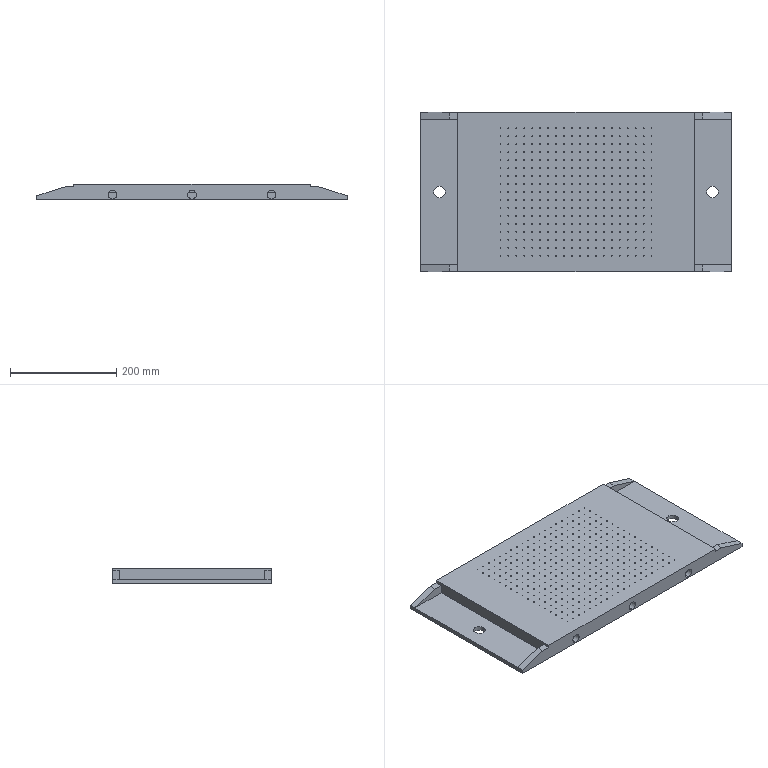Part | STEP file | Platform 2 | 1 solid | 752 faces | box 585 x 300 x 30 mm | volume 2256819 mm3 | cylinder 707 | plane 45 | commonest cylinder face diameters 1.5 x680 10 x9 16.5 x6 20 x4 22 x4 30 x4